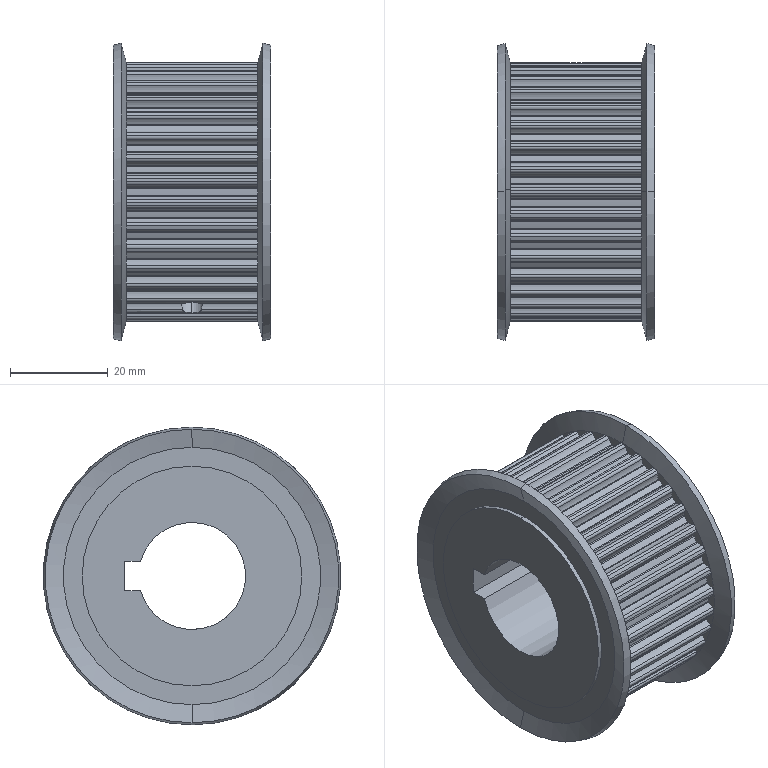Part | STEP file | HTPA34S5M250-A-N22 high-torque timing pulley MISUMI 110 | 1 solid | 382 faces | box 32.194 x 61 x 61 mm | volume 54521 mm3 | cylinder 295 | plane 75 | cone 12 | commonest cylinder face diameters 0.5 x72 1.1 x72 6.55 x72 49.61 x36 53.15 x34 4.917 x4